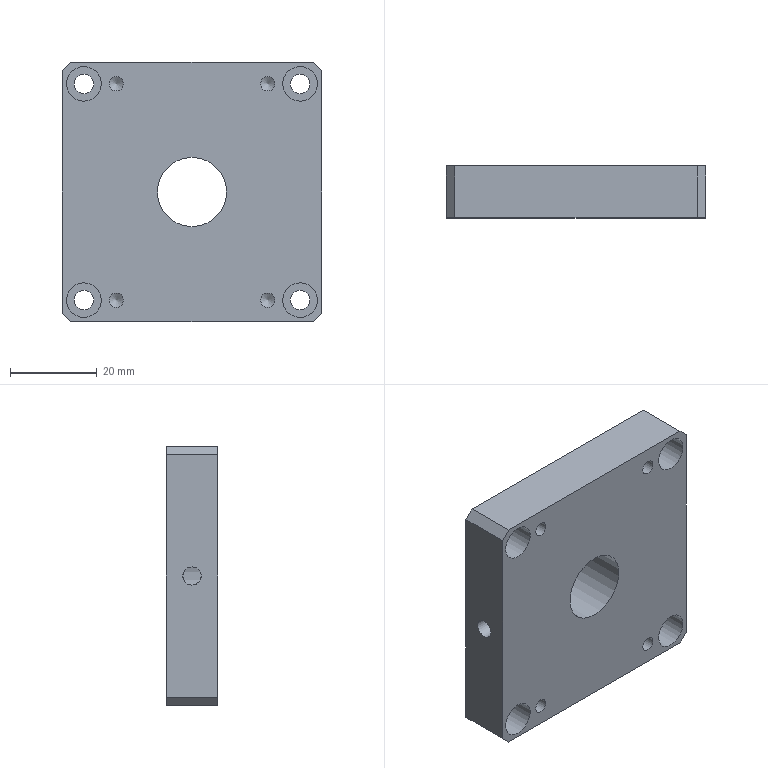Part | NX | 1 solid | 42 faces | box 60 x 12 x 60 mm | volume 38260 mm3 | plane 18 | cylinder 17 | cone 7 | commonest cylinder face diameters 3.3 x4 4.5 x4 8 x4 2 x3 4.2 x1 16 x1
STEP:
#1=CARTESIAN_POINT('',(-30.,6.,2.1));
#2=VERTEX_POINT('',#1);
#3=CARTESIAN_POINT('',(-30.,6.,0.));
#4=DIRECTION('',(-1.,0.,0.));
#5=DIRECTION('',(0.,0.,1.));
#6=AXIS2_PLACEMENT_3D('',#3,#4,#5);
#7=CIRCLE('',#6,2.1);
#8=EDGE_CURVE('',#2,#2,#7,.T.);
#9=ORIENTED_EDGE('',*,*,#8,.T.);
#10=EDGE_LOOP('',(#9));
#11=FACE_BOUND('',#10,.T.);
#12=CARTESIAN_POINT('',(-7.728,6.358,-2.069));
#13=VERTEX_POINT('',#12);
#14=CARTESIAN_POINT('',(-7.932,7.9,-1.344));
#15=CARTESIAN_POINT('',(-7.661,6.398,-2.294));
#16=CARTESIAN_POINT('',(-7.792,4.654,-1.898));
#17=CARTESIAN_POINT('',(-8.057,3.707,-0.4002));
#18=CARTESIAN_POINT('',(-7.932,4.101,1.346));
#19=CARTESIAN_POINT('',(-7.661,5.601,2.292));
#20=CARTESIAN_POINT('',(-7.791,7.344,1.9));
#21=CARTESIAN_POINT('',(-8.057,8.293,0.3983));
#22=CARTESIAN_POINT('',(-7.932,7.9,-1.344));
#23=CARTESIAN_POINT('',(-7.661,6.398,-2.294));
#24=CARTESIAN_POINT('',(-7.792,4.654,-1.898));
#25=B_SPLINE_CURVE_WITH_KNOTS('',3,(#14,#15,#16,#17,#18,#19,#20,#21,#22,#23,#24),.UNSPECIFIED.,.T.,.F.,(1,1,1,1,1,1,1,1,1,1,1,1,1,1,1),(-0.004946,-0.003297,-0.001649,0.,0.001649,0.003297,0.004946,0.006595,0.008243,0.009892,0.01154,0.01319,0.01484,0.01649,0.01814),.UNSPECIFIED.);
#26=EDGE_CURVE('',#13,#13,#25,.T.);
#27=ORIENTED_EDGE('',*,*,#26,.F.);
#28=EDGE_LOOP('',(#27));
#29=FACE_BOUND('',#28,.T.);
#30=CARTESIAN_POINT('',(-30.,6.,0.));
#31=DIRECTION('',(-1.,0.,0.));
#32=DIRECTION('',(0.,0.,1.));
#33=AXIS2_PLACEMENT_3D('',#30,#31,#32);
#34=CYLINDRICAL_SURFACE('',#33,2.1);
#35=ADVANCED_FACE('',(#11,#29),#34,.F.);
#36=CARTESIAN_POINT('',(0.,0.,-8.));
#37=VERTEX_POINT('',#36);
#38=CARTESIAN_POINT('',(0.,0.,0.));
#39=DIRECTION('',(0.,-1.,0.));
#40=DIRECTION('',(0.,0.,-1.));
#41=AXIS2_PLACEMENT_3D('',#38,#39,#40);
#42=CIRCLE('',#41,8.);
#43=EDGE_CURVE('',#37,#37,#42,.F.);
#44=ORIENTED_EDGE('',*,*,#43,.T.);
#45=EDGE_LOOP('',(#44));
#46=FACE_BOUND('',#45,.T.);
#47=CARTESIAN_POINT('',(-30.,0.,-28.));
#48=VERTEX_POINT('',#47);
#49=CARTESIAN_POINT('',(-30.,0.,28.));
#50=VERTEX_POINT('',#49);
#51=CARTESIAN_POINT('',(-30.,0.,30.));
#52=DIRECTION('',(0.,0.,1.));
#53=VECTOR('',#52,1000.);
#54=LINE('',#51,#53);
#55=EDGE_CURVE('',#48,#50,#54,.T.);
#56=ORIENTED_EDGE('',*,*,#55,.F.);
#57=CARTESIAN_POINT('',(-28.,0.,-30.));
#58=VERTEX_POINT('',#57);
#59=CARTESIAN_POINT('',(-29.,0.,-29.));
#60=DIRECTION('',(0.7071,0.,-0.7071));
#61=VECTOR('',#60,1000.);
#62=LINE('',#59,#61);
#63=EDGE_CURVE('',#48,#58,#62,.T.);
#64=ORIENTED_EDGE('',*,*,#63,.T.);
#65=CARTESIAN_POINT('',(28.,0.,-30.));
#66=VERTEX_POINT('',#65);
#67=CARTESIAN_POINT('',(-30.,0.,-30.));
#68=DIRECTION('',(-1.,0.,0.));
#69=VECTOR('',#68,1000.);
#70=LINE('',#67,#69);
#71=EDGE_CURVE('',#66,#58,#70,.T.);
#72=ORIENTED_EDGE('',*,*,#71,.F.);
#73=CARTESIAN_POINT('',(30.,0.,-28.));
#74=VERTEX_POINT('',#73);
#75=CARTESIAN_POINT('',(29.,0.,-29.));
#76=DIRECTION('',(0.7071,0.,0.7071));
#77=VECTOR('',#76,1000.);
#78=LINE('',#75,#77);
#79=EDGE_CURVE('',#66,#74,#78,.T.);
#80=ORIENTED_EDGE('',*,*,#79,.T.);
#81=CARTESIAN_POINT('',(30.,0.,28.));
#82=VERTEX_POINT('',#81);
#83=CARTESIAN_POINT('',(30.,0.,30.));
#84=DIRECTION('',(0.,0.,-1.));
#85=VECTOR('',#84,1000.);
#86=LINE('',#83,#85);
#87=EDGE_CURVE('',#82,#74,#86,.T.);
#88=ORIENTED_EDGE('',*,*,#87,.F.);
#89=CARTESIAN_POINT('',(28.,0.,30.));
#90=VERTEX_POINT('',#89);
#91=CARTESIAN_POINT('',(29.,0.,29.));
#92=DIRECTION('',(-0.7071,0.,0.7071));
#93=VECTOR('',#92,1000.);
#94=LINE('',#91,#93);
#95=EDGE_CURVE('',#82,#90,#94,.T.);
#96=ORIENTED_EDGE('',*,*,#95,.T.);
#97=CARTESIAN_POINT('',(-28.,0.,30.));
#98=VERTEX_POINT('',#97);
#99=CARTESIAN_POINT('',(-30.,0.,30.));
#100=DIRECTION('',(1.,0.,0.));
#101=VECTOR('',#100,1000.);
#102=LINE('',#99,#101);
#103=EDGE_CURVE('',#98,#90,#102,.T.);
#104=ORIENTED_EDGE('',*,*,#103,.F.);
#105=CARTESIAN_POINT('',(-29.,0.,29.));
#106=DIRECTION('',(-0.7071,0.,-0.7071));
#107=VECTOR('',#106,1000.);
#108=LINE('',#105,#107);
#109=EDGE_CURVE('',#98,#50,#108,.T.);
#110=ORIENTED_EDGE('',*,*,#109,.T.);
#111=EDGE_LOOP('',(#56,#64,#72,#80,#88,#96,#104,#110));
#112=FACE_BOUND('',#111,.T.);
#113=CARTESIAN_POINT('',(25.,0.,21.));
#114=VERTEX_POINT('',#113);
#115=CARTESIAN_POINT('',(25.,0.,25.));
#116=DIRECTION('',(0.,-1.,0.));
#117=DIRECTION('',(0.,0.,-1.));
#118=AXIS2_PLACEMENT_3D('',#115,#116,#117);
#119=CIRCLE('',#118,4.);
#120=EDGE_CURVE('',#114,#114,#119,.T.);
#121=ORIENTED_EDGE('',*,*,#120,.F.);
#122=EDGE_LOOP('',(#121));
#123=FACE_BOUND('',#122,.T.);
#124=CARTESIAN_POINT('',(25.,0.,-29.));
#125=VERTEX_POINT('',#124);
#126=CARTESIAN_POINT('',(25.,0.,-25.));
#127=DIRECTION('',(0.,-1.,0.));
#128=DIRECTION('',(0.,0.,-1.));
#129=AXIS2_PLACEMENT_3D('',#126,#127,#128);
#130=CIRCLE('',#129,4.);
#131=EDGE_CURVE('',#125,#125,#130,.T.);
#132=ORIENTED_EDGE('',*,*,#131,.F.);
#133=EDGE_LOOP('',(#132));
#134=FACE_BOUND('',#133,.T.);
#135=CARTESIAN_POINT('',(-25.,0.,-29.));
#136=VERTEX_POINT('',#135);
#137=CARTESIAN_POINT('',(-25.,0.,-25.));
#138=DIRECTION('',(0.,-1.,0.));
#139=DIRECTION('',(0.,0.,-1.));
#140=AXIS2_PLACEMENT_3D('',#137,#138,#139);
#141=CIRCLE('',#140,4.);
#142=EDGE_CURVE('',#136,#136,#141,.T.);
#143=ORIENTED_EDGE('',*,*,#142,.F.);
#144=EDGE_LOOP('',(#143));
#145=FACE_BOUND('',#144,.T.);
#146=CARTESIAN_POINT('',(-25.,0.,21.));
#147=VERTEX_POINT('',#146);
#148=CARTESIAN_POINT('',(-25.,0.,25.));
#149=DIRECTION('',(0.,-1.,0.));
#150=DIRECTION('',(0.,0.,-1.));
#151=AXIS2_PLACEMENT_3D('',#148,#149,#150);
#152=CIRCLE('',#151,4.);
#153=EDGE_CURVE('',#147,#147,#152,.T.);
#154=ORIENTED_EDGE('',*,*,#153,.F.);
#155=EDGE_LOOP('',(#154));
#156=FACE_BOUND('',#155,.T.);
#157=CARTESIAN_POINT('',(17.5,0.,23.35));
#158=VERTEX_POINT('',#157);
#159=CARTESIAN_POINT('',(17.5,0.,25.));
#160=DIRECTION('',(0.,-1.,0.));
#161=DIRECTION('',(0.,0.,-1.));
#162=AXIS2_PLACEMENT_3D('',#159,#160,#161);
#163=CIRCLE('',#162,1.65);
#164=EDGE_CURVE('',#158,#158,#163,.T.);
#165=ORIENTED_EDGE('',*,*,#164,.F.);
#166=EDGE_LOOP('',(#165));
#167=FACE_BOUND('',#166,.T.);
#168=CARTESIAN_POINT('',(17.5,0.,-26.65));
#169=VERTEX_POINT('',#168);
#170=CARTESIAN_POINT('',(17.5,0.,-25.));
#171=DIRECTION('',(0.,-1.,0.));
#172=DIRECTION('',(0.,0.,-1.));
#173=AXIS2_PLACEMENT_3D('',#170,#171,#172);
#174=CIRCLE('',#173,1.65);
#175=EDGE_CURVE('',#169,#169,#174,.T.);
#176=ORIENTED_EDGE('',*,*,#175,.F.);
#177=EDGE_LOOP('',(#176));
#178=FACE_BOUND('',#177,.T.);
#179=CARTESIAN_POINT('',(-17.5,0.,-26.65));
#180=VERTEX_POINT('',#179);
#181=CARTESIAN_POINT('',(-17.5,0.,-25.));
#182=DIRECTION('',(0.,-1.,0.));
#183=DIRECTION('',(0.,0.,-1.));
#184=AXIS2_PLACEMENT_3D('',#181,#182,#183);
#185=CIRCLE('',#184,1.65);
#186=EDGE_CURVE('',#180,#180,#185,.T.);
#187=ORIENTED_EDGE('',*,*,#186,.F.);
#188=EDGE_LOOP('',(#187));
#189=FACE_BOUND('',#188,.T.);
#190=CARTESIAN_POINT('',(-17.5,0.,23.35));
#191=VERTEX_POINT('',#190);
#192=CARTESIAN_POINT('',(-17.5,0.,25.));
#193=DIRECTION('',(0.,-1.,0.));
#194=DIRECTION('',(0.,0.,-1.));
#195=AXIS2_PLACEMENT_3D('',#192,#193,#194);
#196=CIRCLE('',#195,1.65);
#197=EDGE_CURVE('',#191,#191,#196,.T.);
#198=ORIENTED_EDGE('',*,*,#197,.F.);
#199=EDGE_LOOP('',(#198));
#200=FACE_BOUND('',#199,.T.);
#201=CARTESIAN_POINT('',(0.,0.,0.));
#202=DIRECTION('',(0.,-1.,0.));
#203=DIRECTION('',(0.,0.,-1.));
#204=AXIS2_PLACEMENT_3D('',#201,#202,#203);
#205=PLANE('',#204);
#206=ADVANCED_FACE('',(#46,#112,#123,#134,#145,#156,#167,#178,#189,#200),#205,.T.);
#207=CARTESIAN_POINT('',(0.,7.,-24.));
#208=VERTEX_POINT('',#207);
#209=CARTESIAN_POINT('',(0.,7.,-25.));
#210=DIRECTION('',(0.,1.,0.));
#211=DIRECTION('',(0.,0.,1.));
#212=AXIS2_PLACEMENT_3D('',#209,#210,#211);
#213=CIRCLE('',#212,1.);
#214=EDGE_CURVE('',#208,#208,#213,.T.);
#215=ORIENTED_EDGE('',*,*,#214,.T.);
#216=EDGE_LOOP('',(#215));
#217=FACE_BOUND('',#216,.T.);
#218=CARTESIAN_POINT('',(0.,6.399,-25.));
#219=VERTEX_POINT('',#218);
#220=VERTEX_LOOP('',#219);
#221=FACE_BOUND('',#220,.T.);
#222=CARTESIAN_POINT('',(0.,7.,-25.));
#223=DIRECTION('',(0.,1.,0.));
#224=DIRECTION('',(0.,0.,1.));
#225=AXIS2_PLACEMENT_3D('',#222,#223,#224);
#226=CONICAL_SURFACE('',#225,1.,1.03);
#227=ADVANCED_FACE('',(#217,#221),#226,.F.);
#228=CARTESIAN_POINT('',(1.,7.,24.5));
#229=VERTEX_POINT('',#228);
#230=CARTESIAN_POINT('',(0.,6.399,24.5));
#231=VERTEX_POINT('',#230);
#232=CARTESIAN_POINT('',(0.,6.399,24.5));
#233=DIRECTION('',(-0.8572,-0.515,0.));
#234=VECTOR('',#233,1000.);
#235=LINE('',#232,#234);
#236=EDGE_CURVE('',#229,#231,#235,.T.);
#237=ORIENTED_EDGE('',*,*,#236,.F.);
#238=CARTESIAN_POINT('',(-1.,7.,24.5));
#239=VERTEX_POINT('',#238);
#240=CARTESIAN_POINT('',(0.,7.,24.5));
#241=DIRECTION('',(0.,1.,0.));
#242=DIRECTION('',(0.,0.,1.));
#243=AXIS2_PLACEMENT_3D('',#240,#241,#242);
#244=CIRCLE('',#243,1.);
#245=EDGE_CURVE('',#229,#239,#244,.T.);
#246=ORIENTED_EDGE('',*,*,#245,.T.);
#247=CARTESIAN_POINT('',(0.,6.399,24.5));
#248=DIRECTION('',(-0.8572,0.515,0.));
#249=VECTOR('',#248,1000.);
#250=LINE('',#247,#249);
#251=EDGE_CURVE('',#231,#239,#250,.T.);
#252=ORIENTED_EDGE('',*,*,#251,.F.);
#253=EDGE_LOOP('',(#237,#246,#252));
#254=FACE_BOUND('',#253,.T.);
#255=CARTESIAN_POINT('',(0.,7.,24.5));
#256=DIRECTION('',(0.,1.,0.));
#257=DIRECTION('',(0.,0.,1.));
#258=AXIS2_PLACEMENT_3D('',#255,#256,#257);
#259=CONICAL_SURFACE('',#258,1.,1.03);
#260=ADVANCED_FACE('',(#254),#259,.F.);
#261=CARTESIAN_POINT('',(-1.,7.,25.5));
#262=VERTEX_POINT('',#261);
#263=CARTESIAN_POINT('',(-1.,7.,25.5));
#264=DIRECTION('',(0.,0.,-1.));
#265=VECTOR('',#264,1000.);
#266=LINE('',#263,#265);
#267=EDGE_CURVE('',#262,#239,#266,.T.);
#268=ORIENTED_EDGE('',*,*,#267,.F.);
#269=CARTESIAN_POINT('',(0.,6.399,25.5));
#270=VERTEX_POINT('',#269);
#271=CARTESIAN_POINT('',(0.,6.399,25.5));
#272=DIRECTION('',(0.8572,-0.515,0.));
#273=VECTOR('',#272,1000.);
#274=LINE('',#271,#273);
#275=EDGE_CURVE('',#262,#270,#274,.T.);
#276=ORIENTED_EDGE('',*,*,#275,.T.);
#277=CARTESIAN_POINT('',(0.,6.399,25.5));
#278=DIRECTION('',(0.,0.,-1.));
#279=VECTOR('',#278,1000.);
#280=LINE('',#277,#279);
#281=EDGE_CURVE('',#270,#231,#280,.T.);
#282=ORIENTED_EDGE('',*,*,#281,.T.);
#283=ORIENTED_EDGE('',*,*,#251,.T.);
#284=EDGE_LOOP('',(#268,#276,#282,#283));
#285=FACE_BOUND('',#284,.T.);
#286=CARTESIAN_POINT('',(0.,6.399,25.5));
#287=DIRECTION('',(-0.515,-0.8572,0.));
#288=DIRECTION('',(0.8572,-0.515,0.));
#289=AXIS2_PLACEMENT_3D('',#286,#287,#288);
#290=PLANE('',#289);
#291=ADVANCED_FACE('',(#285),#290,.F.);
#292=CARTESIAN_POINT('',(1.,7.,25.5));
#293=VERTEX_POINT('',#292);
#294=CARTESIAN_POINT('',(0.,6.399,25.5));
#295=DIRECTION('',(-0.8572,-0.515,0.));
#296=VECTOR('',#295,1000.);
#297=LINE('',#294,#296);
#298=EDGE_CURVE('',#293,#270,#297,.T.);
#299=ORIENTED_EDGE('',*,*,#298,.T.);
#300=ORIENTED_EDGE('',*,*,#275,.F.);
#301=CARTESIAN_POINT('',(0.,7.,25.5));
#302=DIRECTION('',(0.,1.,0.));
#303=DIRECTION('',(0.,0.,1.));
#304=AXIS2_PLACEMENT_3D('',#301,#302,#303);
#305=CIRCLE('',#304,1.);
#306=EDGE_CURVE('',#262,#293,#305,.T.);
#307=ORIENTED_EDGE('',*,*,#306,.T.);
#308=EDGE_LOOP('',(#299,#300,#307));
#309=FACE_BOUND('',#308,.T.);
#310=CARTESIAN_POINT('',(0.,7.,25.5));
#311=DIRECTION('',(0.,1.,0.));
#312=DIRECTION('',(0.,0.,1.));
#313=AXIS2_PLACEMENT_3D('',#310,#311,#312);
#314=CONICAL_SURFACE('',#313,1.,1.03);
#315=ADVANCED_FACE('',(#309),#314,.F.);
#316=CARTESIAN_POINT('',(1.,7.,25.5));
#317=DIRECTION('',(0.,0.,-1.));
#318=VECTOR('',#317,1000.);
#319=LINE('',#316,#318);
#320=EDGE_CURVE('',#293,#229,#319,.T.);
#321=ORIENTED_EDGE('',*,*,#320,.T.);
#322=ORIENTED_EDGE('',*,*,#236,.T.);
#323=ORIENTED_EDGE('',*,*,#281,.F.);
#324=ORIENTED_EDGE('',*,*,#298,.F.);
#325=EDGE_LOOP('',(#321,#322,#323,#324));
#326=FACE_BOUND('',#325,.T.);
#327=CARTESIAN_POINT('',(0.,6.399,25.5));
#328=DIRECTION('',(0.515,-0.8572,0.));
#329=DIRECTION('',(0.8572,0.515,0.));
#330=AXIS2_PLACEMENT_3D('',#327,#328,#329);
#331=PLANE('',#330);
#332=ADVANCED_FACE('',(#326),#331,.F.);
#333=ORIENTED_EDGE('',*,*,#214,.F.);
#334=EDGE_LOOP('',(#333));
#335=FACE_BOUND('',#334,.T.);
#336=CARTESIAN_POINT('',(0.,12.,-24.));
#337=VERTEX_POINT('',#336);
#338=CARTESIAN_POINT('',(0.,12.,-25.));
#339=DIRECTION('',(0.,1.,0.));
#340=DIRECTION('',(0.,0.,1.));
#341=AXIS2_PLACEMENT_3D('',#338,#339,#340);
#342=CIRCLE('',#341,1.);
#343=EDGE_CURVE('',#337,#337,#342,.T.);
#344=ORIENTED_EDGE('',*,*,#343,.T.);
#345=EDGE_LOOP('',(#344));
#346=FACE_BOUND('',#345,.T.);
#347=CARTESIAN_POINT('',(0.,12.,-25.));
#348=DIRECTION('',(0.,1.,0.));
#349=DIRECTION('',(0.,0.,1.));
#350=AXIS2_PLACEMENT_3D('',#347,#348,#349);
#351=CYLINDRICAL_SURFACE('',#350,1.);
#352=ADVANCED_FACE('',(#335,#346),#351,.F.);
#353=ORIENTED_EDGE('',*,*,#245,.F.);
#354=CARTESIAN_POINT('',(1.,12.,24.5));
#355=VERTEX_POINT('',#354);
#356=CARTESIAN_POINT('',(1.,7.,24.5));
#357=DIRECTION('',(0.,-1.,0.));
#358=VECTOR('',#357,1000.);
#359=LINE('',#356,#358);
#360=EDGE_CURVE('',#355,#229,#359,.T.);
#361=ORIENTED_EDGE('',*,*,#360,.F.);
#362=CARTESIAN_POINT('',(-1.,12.,24.5));
#363=VERTEX_POINT('',#362);
#364=CARTESIAN_POINT('',(0.,12.,24.5));
#365=DIRECTION('',(0.,1.,0.));
#366=DIRECTION('',(0.,0.,1.));
#367=AXIS2_PLACEMENT_3D('',#364,#365,#366);
#368=CIRCLE('',#367,1.);
#369=EDGE_CURVE('',#355,#363,#368,.T.);
#370=ORIENTED_EDGE('',*,*,#369,.T.);
#371=CARTESIAN_POINT('',(-1.,12.,24.5));
#372=DIRECTION('',(0.,1.,0.));
#373=VECTOR('',#372,1000.);
#374=LINE('',#371,#373);
#375=EDGE_CURVE('',#239,#363,#374,.T.);
#376=ORIENTED_EDGE('',*,*,#375,.F.);
#377=EDGE_LOOP('',(#353,#361,#370,#376));
#378=FACE_BOUND('',#377,.T.);
#379=CARTESIAN_POINT('',(0.,12.,24.5));
#380=DIRECTION('',(0.,1.,0.));
#381=DIRECTION('',(0.,0.,1.));
#382=AXIS2_PLACEMENT_3D('',#379,#380,#381);
#383=CYLINDRICAL_SURFACE('',#382,1.);
#384=ADVANCED_FACE('',(#378),#383,.F.);
#385=CARTESIAN_POINT('',(-1.,12.,25.5));
#386=VERTEX_POINT('',#385);
#387=CARTESIAN_POINT('',(-1.,12.,25.5));
#388=DIRECTION('',(0.,0.,-1.));
#389=VECTOR('',#388,1000.);
#390=LINE('',#387,#389);
#391=EDGE_CURVE('',#386,#363,#390,.T.);
#392=ORIENTED_EDGE('',*,*,#391,.F.);
#393=CARTESIAN_POINT('',(-1.,12.,25.5));
#394=DIRECTION('',(0.,-1.,0.));
#395=VECTOR('',#394,1000.);
#396=LINE('',#393,#395);
#397=EDGE_CURVE('',#386,#262,#396,.T.);
#398=ORIENTED_EDGE('',*,*,#397,.T.);
#399=ORIENTED_EDGE('',*,*,#267,.T.);
#400=ORIENTED_EDGE('',*,*,#375,.T.);
#401=EDGE_LOOP('',(#392,#398,#399,#400));
#402=FACE_BOUND('',#401,.T.);
#403=CARTESIAN_POINT('',(-1.,12.,25.5));
#404=DIRECTION('',(-1.,0.,0.));
#405=DIRECTION('',(0.,0.,1.));
#406=AXIS2_PLACEMENT_3D('',#403,#404,#405);
#407=PLANE('',#406);
#408=ADVANCED_FACE('',(#402),#407,.F.);
#409=ORIENTED_EDGE('',*,*,#306,.F.);
#410=ORIENTED_EDGE('',*,*,#397,.F.);
#411=CARTESIAN_POINT('',(1.,12.,25.5));
#412=VERTEX_POINT('',#411);
#413=CARTESIAN_POINT('',(0.,12.,25.5));
#414=DIRECTION('',(0.,1.,0.));
#415=DIRECTION('',(0.,0.,1.));
#416=AXIS2_PLACEMENT_3D('',#413,#414,#415);
#417=CIRCLE('',#416,1.);
#418=EDGE_CURVE('',#386,#412,#417,.T.);
#419=ORIENTED_EDGE('',*,*,#418,.T.);
#420=CARTESIAN_POINT('',(1.,7.,25.5));
#421=DIRECTION('',(0.,-1.,0.));
#422=VECTOR('',#421,1000.);
#423=LINE('',#420,#422);
#424=EDGE_CURVE('',#412,#293,#423,.T.);
#425=ORIENTED_EDGE('',*,*,#424,.T.);
#426=EDGE_LOOP('',(#409,#410,#419,#425));
#427=FACE_BOUND('',#426,.T.);
#428=CARTESIAN_POINT('',(0.,12.,25.5));
#429=DIRECTION('',(0.,1.,0.));
#430=DIRECTION('',(0.,0.,1.));
#431=AXIS2_PLACEMENT_3D('',#428,#429,#430);
#432=CYLINDRICAL_SURFACE('',#431,1.);
#433=ADVANCED_FACE('',(#427),#432,.F.);
#434=CARTESIAN_POINT('',(1.,12.,25.5));
#435=DIRECTION('',(0.,0.,-1.));
#436=VECTOR('',#435,1000.);
#437=LINE('',#434,#436);
#438=EDGE_CURVE('',#412,#355,#437,.T.);
#439=ORIENTED_EDGE('',*,*,#438,.T.);
#440=ORIENTED_EDGE('',*,*,#360,.T.);
#441=ORIENTED_EDGE('',*,*,#320,.F.);
#442=ORIENTED_EDGE('',*,*,#424,.F.);
#443=EDGE_LOOP('',(#439,#440,#441,#442));
#444=FACE_BOUND('',#443,.T.);
#445=CARTESIAN_POINT('',(1.,7.,25.5));
#446=DIRECTION('',(1.,0.,0.));
#447=DIRECTION('',(0.,1.,0.));
#448=AXIS2_PLACEMENT_3D('',#445,#446,#447);
#449=PLANE('',#448);
#450=ADVANCED_FACE('',(#444),#449,.F.);
#451=CARTESIAN_POINT('',(-25.,7.,22.75));
#452=VERTEX_POINT('',#451);
#453=CARTESIAN_POINT('',(-25.,7.,25.));
#454=DIRECTION('',(0.,-1.,0.));
#455=DIRECTION('',(0.,0.,-1.));
#456=AXIS2_PLACEMENT_3D('',#453,#454,#455);
#457=CIRCLE('',#456,2.25);
#458=EDGE_CURVE('',#452,#452,#457,.T.);
#459=ORIENTED_EDGE('',*,*,#458,.T.);
#460=EDGE_LOOP('',(#459));
#461=FACE_BOUND('',#460,.T.);
#462=CARTESIAN_POINT('',(-25.,12.,22.75));
#463=VERTEX_POINT('',#462);
#464=CARTESIAN_POINT('',(-25.,12.,25.));
#465=DIRECTION('',(0.,-1.,0.));
#466=DIRECTION('',(0.,0.,-1.));
#467=AXIS2_PLACEMENT_3D('',#464,#465,#466);
#468=CIRCLE('',#467,2.25);
#469=EDGE_CURVE('',#463,#463,#468,.T.);
#470=ORIENTED_EDGE('',*,*,#469,.F.);
#471=EDGE_LOOP('',(#470));
#472=FACE_BOUND('',#471,.T.);
#473=CARTESIAN_POINT('',(-25.,0.,25.));
#474=DIRECTION('',(0.,-1.,0.));
#475=DIRECTION('',(0.,0.,-1.));
#476=AXIS2_PLACEMENT_3D('',#473,#474,#475);
#477=CYLINDRICAL_SURFACE('',#476,2.25);
#478=ADVANCED_FACE('',(#461,#472),#477,.F.);
#479=CARTESIAN_POINT('',(-25.,7.,-22.75));
#480=VERTEX_POINT('',#479);
#481=CARTESIAN_POINT('',(-25.,7.,-25.));
#482=DIRECTION('',(0.,-1.,0.));
#483=DIRECTION('',(0.,0.,1.));
#484=AXIS2_PLACEMENT_3D('',#481,#482,#483);
#485=CIRCLE('',#484,2.25);
#486=EDGE_CURVE('',#480,#480,#485,.T.);
#487=ORIENTED_EDGE('',*,*,#486,.T.);
#488=EDGE_LOOP('',(#487));
#489=FACE_BOUND('',#488,.T.);
#490=CARTESIAN_POINT('',(-25.,12.,-27.25));
#491=VERTEX_POINT('',#490);
#492=CARTESIAN_POINT('',(-25.,12.,-25.));
#493=DIRECTION('',(0.,-1.,0.));
#494=DIRECTION('',(0.,0.,-1.));
#495=AXIS2_PLACEMENT_3D('',#492,#493,#494);
#496=CIRCLE('',#495,2.25);
#497=EDGE_CURVE('',#491,#491,#496,.T.);
#498=ORIENTED_EDGE('',*,*,#497,.F.);
#499=EDGE_LOOP('',(#498));
#500=FACE_BOUND('',#499,.T.);
#501=CARTESIAN_POINT('',(-25.,0.,-25.));
#502=DIRECTION('',(0.,-1.,0.));
#503=DIRECTION('',(0.,0.,-1.));
#504=AXIS2_PLACEMENT_3D('',#501,#502,#503);
#505=CYLINDRICAL_SURFACE('',#504,2.25);
#506=ADVANCED_FACE('',(#489,#500),#505,.F.);
#507=CARTESIAN_POINT('',(25.,7.,-22.75));
#508=VERTEX_POINT('',#507);
#509=CARTESIAN_POINT('',(25.,7.,-25.));
#510=DIRECTION('',(0.,-1.,0.));
#511=DIRECTION('',(0.,0.,1.));
#512=AXIS2_PLACEMENT_3D('',#509,#510,#511);
#513=CIRCLE('',#512,2.25);
#514=EDGE_CURVE('',#508,#508,#513,.T.);
#515=ORIENTED_EDGE('',*,*,#514,.T.);
#516=EDGE_LOOP('',(#515));
#517=FACE_BOUND('',#516,.T.);
#518=CARTESIAN_POINT('',(25.,12.,-27.25));
#519=VERTEX_POINT('',#518);
#520=CARTESIAN_POINT('',(25.,12.,-25.));
#521=DIRECTION('',(0.,-1.,0.));
#522=DIRECTION('',(0.,0.,-1.));
#523=AXIS2_PLACEMENT_3D('',#520,#521,#522);
#524=CIRCLE('',#523,2.25);
#525=EDGE_CURVE('',#519,#519,#524,.T.);
#526=ORIENTED_EDGE('',*,*,#525,.F.);
#527=EDGE_LOOP('',(#526));
#528=FACE_BOUND('',#527,.T.);
#529=CARTESIAN_POINT('',(25.,0.,-25.));
#530=DIRECTION('',(0.,-1.,0.));
#531=DIRECTION('',(0.,0.,-1.));
#532=AXIS2_PLACEMENT_3D('',#529,#530,#531);
#533=CYLINDRICAL_SURFACE('',#532,2.25);
#534=ADVANCED_FACE('',(#517,#528),#533,.F.);
#535=CARTESIAN_POINT('',(25.,7.,27.25));
#536=VERTEX_POINT('',#535);
#537=CARTESIAN_POINT('',(25.,7.,25.));
#538=DIRECTION('',(0.,-1.,0.));
#539=DIRECTION('',(0.,0.,1.));
#540=AXIS2_PLACEMENT_3D('',#537,#538,#539);
#541=CIRCLE('',#540,2.25);
#542=EDGE_CURVE('',#536,#536,#541,.T.);
#543=ORIENTED_EDGE('',*,*,#542,.T.);
#544=EDGE_LOOP('',(#543));
#545=FACE_BOUND('',#544,.T.);
#546=CARTESIAN_POINT('',(25.,12.,22.75));
#547=VERTEX_POINT('',#546);
#548=CARTESIAN_POINT('',(25.,12.,25.));
#549=DIRECTION('',(0.,-1.,0.));
#550=DIRECTION('',(0.,0.,-1.));
#551=AXIS2_PLACEMENT_3D('',#548,#549,#550);
#552=CIRCLE('',#551,2.25);
#553=EDGE_CURVE('',#547,#547,#552,.T.);
#554=ORIENTED_EDGE('',*,*,#553,.F.);
#555=EDGE_LOOP('',(#554));
#556=FACE_BOUND('',#555,.T.);
#557=CARTESIAN_POINT('',(25.,0.,25.));
#558=DIRECTION('',(0.,-1.,0.));
#559=DIRECTION('',(0.,0.,-1.));
#560=AXIS2_PLACEMENT_3D('',#557,#558,#559);
#561=CYLINDRICAL_SURFACE('',#560,2.25);
#562=ADVANCED_FACE('',(#545,#556),#561,.F.);
#563=CARTESIAN_POINT('',(-17.5,11.091,25.));
#564=VERTEX_POINT('',#563);
#565=VERTEX_LOOP('',#564);
#566=FACE_BOUND('',#565,.T.);
#567=CARTESIAN_POINT('',(-17.5,10.1,23.35));
#568=VERTEX_POINT('',#567);
#569=CARTESIAN_POINT('',(-17.5,10.1,25.));
#570=DIRECTION('',(0.,-1.,0.));
#571=DIRECTION('',(0.,0.,-1.));
#572=AXIS2_PLACEMENT_3D('',#569,#570,#571);
#573=CIRCLE('',#572,1.65);
#574=EDGE_CURVE('',#568,#568,#573,.T.);
#575=ORIENTED_EDGE('',*,*,#574,.T.);
#576=EDGE_LOOP('',(#575));
#577=FACE_BOUND('',#576,.T.);
#578=CARTESIAN_POINT('',(-17.5,10.1,25.));
#579=DIRECTION('',(0.,-1.,0.));
#580=DIRECTION('',(0.,0.,-1.));
#581=AXIS2_PLACEMENT_3D('',#578,#579,#580);
#582=CONICAL_SURFACE('',#581,1.65,1.03);
#583=ADVANCED_FACE('',(#566,#577),#582,.F.);
#584=CARTESIAN_POINT('',(-17.5,11.091,-25.));
#585=VERTEX_POINT('',#584);
#586=VERTEX_LOOP('',#585);
#587=FACE_BOUND('',#586,.T.);
#588=CARTESIAN_POINT('',(-17.5,10.1,-26.65));
#589=VERTEX_POINT('',#588);
#590=CARTESIAN_POINT('',(-17.5,10.1,-25.));
#591=DIRECTION('',(0.,-1.,0.));
#592=DIRECTION('',(0.,0.,-1.));
#593=AXIS2_PLACEMENT_3D('',#590,#591,#592);
#594=CIRCLE('',#593,1.65);
#595=EDGE_CURVE('',#589,#589,#594,.T.);
#596=ORIENTED_EDGE('',*,*,#595,.T.);
#597=EDGE_LOOP('',(#596));
#598=FACE_BOUND('',#597,.T.);
#599=CARTESIAN_POINT('',(-17.5,10.1,-25.));
#600=DIRECTION('',(0.,-1.,0.));
#601=DIRECTION('',(0.,0.,-1.));
#602=AXIS2_PLACEMENT_3D('',#599,#600,#601);
#603=CONICAL_SURFACE('',#602,1.65,1.03);
#604=ADVANCED_FACE('',(#587,#598),#603,.F.);
#605=CARTESIAN_POINT('',(17.5,11.091,-25.));
#606=VERTEX_POINT('',#605);
#607=VERTEX_LOOP('',#606);
#608=FACE_BOUND('',#607,.T.);
#609=CARTESIAN_POINT('',(17.5,10.1,-26.65));
#610=VERTEX_POINT('',#609);
#611=CARTESIAN_POINT('',(17.5,10.1,-25.));
#612=DIRECTION('',(0.,-1.,0.));
#613=DIRECTION('',(0.,0.,-1.));
#614=AXIS2_PLACEMENT_3D('',#611,#612,#613);
#615=CIRCLE('',#614,1.65);
#616=EDGE_CURVE('',#610,#610,#615,.T.);
#617=ORIENTED_EDGE('',*,*,#616,.T.);
#618=EDGE_LOOP('',(#617));
#619=FACE_BOUND('',#618,.T.);
#620=CARTESIAN_POINT('',(17.5,10.1,-25.));
#621=DIRECTION('',(0.,-1.,0.));
#622=DIRECTION('',(0.,0.,-1.));
#623=AXIS2_PLACEMENT_3D('',#620,#621,#622);
#624=CONICAL_SURFACE('',#623,1.65,1.03);
#625=ADVANCED_FACE('',(#608,#619),#624,.F.);
#626=CARTESIAN_POINT('',(17.5,11.091,25.));
#627=VERTEX_POINT('',#626);
#628=VERTEX_LOOP('',#627);
#629=FACE_BOUND('',#628,.T.);
#630=CARTESIAN_POINT('',(17.5,10.1,23.35));
#631=VERTEX_POINT('',#630);
#632=CARTESIAN_POINT('',(17.5,10.1,25.));
#633=DIRECTION('',(0.,-1.,0.));
#634=DIRECTION('',(0.,0.,-1.));
#635=AXIS2_PLACEMENT_3D('',#632,#633,#634);
#636=CIRCLE('',#635,1.65);
#637=EDGE_CURVE('',#631,#631,#636,.T.);
#638=ORIENTED_EDGE('',*,*,#637,.T.);
#639=EDGE_LOOP('',(#638));
#640=FACE_BOUND('',#639,.T.);
#641=CARTESIAN_POINT('',(17.5,10.1,25.));
#642=DIRECTION('',(0.,-1.,0.));
#643=DIRECTION('',(0.,0.,-1.));
#644=AXIS2_PLACEMENT_3D('',#641,#642,#643);
#645=CONICAL_SURFACE('',#644,1.65,1.03);
#646=ADVANCED_FACE('',(#629,#640),#645,.F.);
#647=CARTESIAN_POINT('',(-25.,7.,21.));
#648=VERTEX_POINT('',#647);
#649=CARTESIAN_POINT('',(-25.,7.,25.));
#650=DIRECTION('',(0.,-1.,0.));
#651=DIRECTION('',(0.,0.,-1.));
#652=AXIS2_PLACEMENT_3D('',#649,#650,#651);
#653=CIRCLE('',#652,4.);
#654=EDGE_CURVE('',#648,#648,#653,.T.);
#655=ORIENTED_EDGE('',*,*,#654,.T.);
#656=EDGE_LOOP('',(#655));
#657=FACE_BOUND('',#656,.T.);
#658=ORIENTED_EDGE('',*,*,#458,.F.);
#659=EDGE_LOOP('',(#658));
#660=FACE_BOUND('',#659,.T.);
#661=CARTESIAN_POINT('',(-22.75,7.,25.));
#662=DIRECTION('',(0.,1.,0.));
#663=DIRECTION('',(0.,0.,1.));
#664=AXIS2_PLACEMENT_3D('',#661,#662,#663);
#665=PLANE('',#664);
#666=ADVANCED_FACE('',(#657,#660),#665,.F.);
#667=CARTESIAN_POINT('',(-25.,7.,-21.));
#668=VERTEX_POINT('',#667);
#669=CARTESIAN_POINT('',(-25.,7.,-25.));
#670=DIRECTION('',(0.,-1.,0.));
#671=DIRECTION('',(0.,0.,1.));
#672=AXIS2_PLACEMENT_3D('',#669,#670,#671);
#673=CIRCLE('',#672,4.);
#674=EDGE_CURVE('',#668,#668,#673,.T.);
#675=ORIENTED_EDGE('',*,*,#674,.T.);
#676=EDGE_LOOP('',(#675));
#677=FACE_BOUND('',#676,.T.);
#678=ORIENTED_EDGE('',*,*,#486,.F.);
#679=EDGE_LOOP('',(#678));
#680=FACE_BOUND('',#679,.T.);
#681=CARTESIAN_POINT('',(-22.75,7.,25.));
#682=DIRECTION('',(0.,1.,0.));
#683=DIRECTION('',(0.,0.,1.));
#684=AXIS2_PLACEMENT_3D('',#681,#682,#683);
#685=PLANE('',#684);
#686=ADVANCED_FACE('',(#677,#680),#685,.F.);
#687=CARTESIAN_POINT('',(25.,7.,-21.));
#688=VERTEX_POINT('',#687);
#689=CARTESIAN_POINT('',(25.,7.,-25.));
#690=DIRECTION('',(0.,-1.,0.));
#691=DIRECTION('',(0.,0.,1.));
#692=AXIS2_PLACEMENT_3D('',#689,#690,#691);
#693=CIRCLE('',#692,4.);
#694=EDGE_CURVE('',#688,#688,#693,.T.);
#695=ORIENTED_EDGE('',*,*,#694,.T.);
#696=EDGE_LOOP('',(#695));
#697=FACE_BOUND('',#696,.T.);
#698=ORIENTED_EDGE('',*,*,#514,.F.);
#699=EDGE_LOOP('',(#698));
#700=FACE_BOUND('',#699,.T.);
#701=CARTESIAN_POINT('',(-22.75,7.,25.));
#702=DIRECTION('',(0.,1.,0.));
#703=DIRECTION('',(0.,0.,1.));
#704=AXIS2_PLACEMENT_3D('',#701,#702,#703);
#705=PLANE('',#704);
#706=ADVANCED_FACE('',(#697,#700),#705,.F.);
#707=CARTESIAN_POINT('',(25.,7.,29.));
#708=VERTEX_POINT('',#707);
#709=CARTESIAN_POINT('',(25.,7.,25.));
#710=DIRECTION('',(0.,-1.,0.));
#711=DIRECTION('',(0.,0.,1.));
#712=AXIS2_PLACEMENT_3D('',#709,#710,#711);
#713=CIRCLE('',#712,4.);
#714=EDGE_CURVE('',#708,#708,#713,.T.);
#715=ORIENTED_EDGE('',*,*,#714,.T.);
#716=EDGE_LOOP('',(#715));
#717=FACE_BOUND('',#716,.T.);
#718=ORIENTED_EDGE('',*,*,#542,.F.);
#719=EDGE_LOOP('',(#718));
#720=FACE_BOUND('',#719,.T.);
#721=CARTESIAN_POINT('',(-22.75,7.,25.));
#722=DIRECTION('',(0.,1.,0.));
#723=DIRECTION('',(0.,0.,1.));
#724=AXIS2_PLACEMENT_3D('',#721,#722,#723);
#725=PLANE('',#724);
#726=ADVANCED_FACE('',(#717,#720),#725,.F.);
#727=CARTESIAN_POINT('',(0.,12.,-8.));
#728=VERTEX_POINT('',#727);
#729=CARTESIAN_POINT('',(0.,12.,0.));
#730=DIRECTION('',(0.,-1.,0.));
#731=DIRECTION('',(0.,0.,-1.));
#732=AXIS2_PLACEMENT_3D('',#729,#730,#731);
#733=CIRCLE('',#732,8.);
#734=EDGE_CURVE('',#728,#728,#733,.F.);
#735=ORIENTED_EDGE('',*,*,#734,.F.);
#736=EDGE_LOOP('',(#735));
#737=FACE_BOUND('',#736,.T.);
#738=CARTESIAN_POINT('',(28.,12.,-30.));
#739=VERTEX_POINT('',#738);
#740=CARTESIAN_POINT('',(-28.,12.,-30.));
#741=VERTEX_POINT('',#740);
#742=CARTESIAN_POINT('',(-30.,12.,-30.));
#743=DIRECTION('',(-1.,0.,0.));
#744=VECTOR('',#743,1000.);
#745=LINE('',#742,#744);
#746=EDGE_CURVE('',#739,#741,#745,.T.);
#747=ORIENTED_EDGE('',*,*,#746,.T.);
#748=CARTESIAN_POINT('',(-30.,12.,-28.));
#749=VERTEX_POINT('',#748);
#750=CARTESIAN_POINT('',(-30.,12.,-28.));
#751=DIRECTION('',(-0.7071,0.,0.7071));
#752=VECTOR('',#751,1000.);
#753=LINE('',#750,#752);
#754=EDGE_CURVE('',#741,#749,#753,.T.);
#755=ORIENTED_EDGE('',*,*,#754,.T.);
#756=CARTESIAN_POINT('',(-30.,12.,28.));
#757=VERTEX_POINT('',#756);
#758=CARTESIAN_POINT('',(-30.,12.,30.));
#759=DIRECTION('',(0.,0.,1.));
#760=VECTOR('',#759,1000.);
#761=LINE('',#758,#760);
#762=EDGE_CURVE('',#749,#757,#761,.T.);
#763=ORIENTED_EDGE('',*,*,#762,.T.);
#764=CARTESIAN_POINT('',(-28.,12.,30.));
#765=VERTEX_POINT('',#764);
#766=CARTESIAN_POINT('',(-28.,12.,30.));
#767=DIRECTION('',(0.7071,0.,0.7071));
#768=VECTOR('',#767,1000.);
#769=LINE('',#766,#768);
#770=EDGE_CURVE('',#757,#765,#769,.T.);
#771=ORIENTED_EDGE('',*,*,#770,.T.);
#772=CARTESIAN_POINT('',(28.,12.,30.));
#773=VERTEX_POINT('',#772);
#774=CARTESIAN_POINT('',(-30.,12.,30.));
#775=DIRECTION('',(1.,0.,0.));
#776=VECTOR('',#775,1000.);
#777=LINE('',#774,#776);
#778=EDGE_CURVE('',#765,#773,#777,.T.);
#779=ORIENTED_EDGE('',*,*,#778,.T.);
#780=CARTESIAN_POINT('',(30.,12.,28.));
#781=VERTEX_POINT('',#780);
#782=CARTESIAN_POINT('',(30.,12.,28.));
#783=DIRECTION('',(0.7071,0.,-0.7071));
#784=VECTOR('',#783,1000.);
#785=LINE('',#782,#784);
#786=EDGE_CURVE('',#773,#781,#785,.T.);
#787=ORIENTED_EDGE('',*,*,#786,.T.);
#788=CARTESIAN_POINT('',(30.,12.,-28.));
#789=VERTEX_POINT('',#788);
#790=CARTESIAN_POINT('',(30.,12.,30.));
#791=DIRECTION('',(0.,0.,-1.));
#792=VECTOR('',#791,1000.);
#793=LINE('',#790,#792);
#794=EDGE_CURVE('',#781,#789,#793,.T.);
#795=ORIENTED_EDGE('',*,*,#794,.T.);
#796=CARTESIAN_POINT('',(28.,12.,-30.));
#797=DIRECTION('',(-0.7071,0.,-0.7071));
#798=VECTOR('',#797,1000.);
#799=LINE('',#796,#798);
#800=EDGE_CURVE('',#789,#739,#799,.T.);
#801=ORIENTED_EDGE('',*,*,#800,.T.);
#802=EDGE_LOOP('',(#747,#755,#763,#771,#779,#787,#795,#801));
#803=FACE_BOUND('',#802,.T.);
#804=ORIENTED_EDGE('',*,*,#553,.T.);
#805=EDGE_LOOP('',(#804));
#806=FACE_BOUND('',#805,.T.);
#807=ORIENTED_EDGE('',*,*,#525,.T.);
#808=EDGE_LOOP('',(#807));
#809=FACE_BOUND('',#808,.T.);
#810=ORIENTED_EDGE('',*,*,#497,.T.);
#811=EDGE_LOOP('',(#810));
#812=FACE_BOUND('',#811,.T.);
#813=ORIENTED_EDGE('',*,*,#469,.T.);
#814=EDGE_LOOP('',(#813));
#815=FACE_BOUND('',#814,.T.);
#816=ORIENTED_EDGE('',*,*,#438,.F.);
#817=ORIENTED_EDGE('',*,*,#418,.F.);
#818=ORIENTED_EDGE('',*,*,#391,.T.);
#819=ORIENTED_EDGE('',*,*,#369,.F.);
#820=EDGE_LOOP('',(#816,#817,#818,#819));
#821=FACE_BOUND('',#820,.T.);
#822=ORIENTED_EDGE('',*,*,#343,.F.);
#823=EDGE_LOOP('',(#822));
#824=FACE_BOUND('',#823,.T.);
#825=CARTESIAN_POINT('',(0.,12.,0.));
#826=DIRECTION('',(0.,-1.,0.));
#827=DIRECTION('',(0.,0.,-1.));
#828=AXIS2_PLACEMENT_3D('',#825,#826,#827);
#829=PLANE('',#828);
#830=ADVANCED_FACE('',(#737,#803,#806,#809,#812,#815,#821,#824),#829,.F.);
#831=ORIENTED_EDGE('',*,*,#197,.T.);
#832=EDGE_LOOP('',(#831));
#833=FACE_BOUND('',#832,.T.);
#834=ORIENTED_EDGE('',*,*,#574,.F.);
#835=EDGE_LOOP('',(#834));
#836=FACE_BOUND('',#835,.T.);
#837=CARTESIAN_POINT('',(-17.5,0.,25.));
#838=DIRECTION('',(0.,-1.,0.));
#839=DIRECTION('',(0.,0.,-1.));
#840=AXIS2_PLACEMENT_3D('',#837,#838,#839);
#841=CYLINDRICAL_SURFACE('',#840,1.65);
#842=ADVANCED_FACE('',(#833,#836),#841,.F.);
#843=ORIENTED_EDGE('',*,*,#186,.T.);
#844=EDGE_LOOP('',(#843));
#845=FACE_BOUND('',#844,.T.);
#846=ORIENTED_EDGE('',*,*,#595,.F.);
#847=EDGE_LOOP('',(#846));
#848=FACE_BOUND('',#847,.T.);
#849=CARTESIAN_POINT('',(-17.5,0.,-25.));
#850=DIRECTION('',(0.,-1.,0.));
#851=DIRECTION('',(0.,0.,-1.));
#852=AXIS2_PLACEMENT_3D('',#849,#850,#851);
#853=CYLINDRICAL_SURFACE('',#852,1.65);
#854=ADVANCED_FACE('',(#845,#848),#853,.F.);
#855=ORIENTED_EDGE('',*,*,#175,.T.);
#856=EDGE_LOOP('',(#855));
#857=FACE_BOUND('',#856,.T.);
#858=ORIENTED_EDGE('',*,*,#616,.F.);
#859=EDGE_LOOP('',(#858));
#860=FACE_BOUND('',#859,.T.);
#861=CARTESIAN_POINT('',(17.5,0.,-25.));
#862=DIRECTION('',(0.,-1.,0.));
#863=DIRECTION('',(0.,0.,-1.));
#864=AXIS2_PLACEMENT_3D('',#861,#862,#863);
#865=CYLINDRICAL_SURFACE('',#864,1.65);
#866=ADVANCED_FACE('',(#857,#860),#865,.F.);
#867=ORIENTED_EDGE('',*,*,#164,.T.);
#868=EDGE_LOOP('',(#867));
#869=FACE_BOUND('',#868,.T.);
#870=ORIENTED_EDGE('',*,*,#637,.F.);
#871=EDGE_LOOP('',(#870));
#872=FACE_BOUND('',#871,.T.);
#873=CARTESIAN_POINT('',(17.5,0.,25.));
#874=DIRECTION('',(0.,-1.,0.));
#875=DIRECTION('',(0.,0.,-1.));
#876=AXIS2_PLACEMENT_3D('',#873,#874,#875);
#877=CYLINDRICAL_SURFACE('',#876,1.65);
#878=ADVANCED_FACE('',(#869,#872),#877,.F.);
#879=ORIENTED_EDGE('',*,*,#153,.T.);
#880=EDGE_LOOP('',(#879));
#881=FACE_BOUND('',#880,.T.);
#882=ORIENTED_EDGE('',*,*,#654,.F.);
#883=EDGE_LOOP('',(#882));
#884=FACE_BOUND('',#883,.T.);
#885=CARTESIAN_POINT('',(-25.,0.,25.));
#886=DIRECTION('',(0.,-1.,0.));
#887=DIRECTION('',(0.,0.,-1.));
#888=AXIS2_PLACEMENT_3D('',#885,#886,#887);
#889=CYLINDRICAL_SURFACE('',#888,4.);
#890=ADVANCED_FACE('',(#881,#884),#889,.F.);
#891=ORIENTED_EDGE('',*,*,#142,.T.);
#892=EDGE_LOOP('',(#891));
#893=FACE_BOUND('',#892,.T.);
#894=ORIENTED_EDGE('',*,*,#674,.F.);
#895=EDGE_LOOP('',(#894));
#896=FACE_BOUND('',#895,.T.);
#897=CARTESIAN_POINT('',(-25.,0.,-25.));
#898=DIRECTION('',(0.,-1.,0.));
#899=DIRECTION('',(0.,0.,-1.));
#900=AXIS2_PLACEMENT_3D('',#897,#898,#899);
#901=CYLINDRICAL_SURFACE('',#900,4.);
#902=ADVANCED_FACE('',(#893,#896),#901,.F.);
#903=ORIENTED_EDGE('',*,*,#131,.T.);
#904=EDGE_LOOP('',(#903));
#905=FACE_BOUND('',#904,.T.);
#906=ORIENTED_EDGE('',*,*,#694,.F.);
#907=EDGE_LOOP('',(#906));
#908=FACE_BOUND('',#907,.T.);
#909=CARTESIAN_POINT('',(25.,0.,-25.));
#910=DIRECTION('',(0.,-1.,0.));
#911=DIRECTION('',(0.,0.,-1.));
#912=AXIS2_PLACEMENT_3D('',#909,#910,#911);
#913=CYLINDRICAL_SURFACE('',#912,4.);
#914=ADVANCED_FACE('',(#905,#908),#913,.F.);
#915=ORIENTED_EDGE('',*,*,#120,.T.);
#916=EDGE_LOOP('',(#915));
#917=FACE_BOUND('',#916,.T.);
#918=ORIENTED_EDGE('',*,*,#714,.F.);
#919=EDGE_LOOP('',(#918));
#920=FACE_BOUND('',#919,.T.);
#921=CARTESIAN_POINT('',(25.,0.,25.));
#922=DIRECTION('',(0.,-1.,0.));
#923=DIRECTION('',(0.,0.,-1.));
#924=AXIS2_PLACEMENT_3D('',#921,#922,#923);
#925=CYLINDRICAL_SURFACE('',#924,4.);
#926=ADVANCED_FACE('',(#917,#920),#925,.F.);
#927=ORIENTED_EDGE('',*,*,#770,.F.);
#928=CARTESIAN_POINT('',(-30.,12.,28.));
#929=DIRECTION('',(0.,1.,0.));
#930=VECTOR('',#929,1000.);
#931=LINE('',#928,#930);
#932=EDGE_CURVE('',#50,#757,#931,.T.);
#933=ORIENTED_EDGE('',*,*,#932,.F.);
#934=ORIENTED_EDGE('',*,*,#109,.F.);
#935=CARTESIAN_POINT('',(-28.,12.,30.));
#936=DIRECTION('',(0.,-1.,0.));
#937=VECTOR('',#936,1000.);
#938=LINE('',#935,#937);
#939=EDGE_CURVE('',#765,#98,#938,.T.);
#940=ORIENTED_EDGE('',*,*,#939,.F.);
#941=EDGE_LOOP('',(#927,#933,#934,#940));
#942=FACE_BOUND('',#941,.T.);
#943=CARTESIAN_POINT('',(-28.,12.,30.));
#944=DIRECTION('',(0.7071,0.,-0.7071));
#945=DIRECTION('',(0.,-1.,0.));
#946=AXIS2_PLACEMENT_3D('',#943,#944,#945);
#947=PLANE('',#946);
#948=ADVANCED_FACE('',(#942),#947,.F.);
#949=ORIENTED_EDGE('',*,*,#103,.T.);
#950=CARTESIAN_POINT('',(28.,12.,30.));
#951=DIRECTION('',(0.,1.,0.));
#952=VECTOR('',#951,1000.);
#953=LINE('',#950,#952);
#954=EDGE_CURVE('',#90,#773,#953,.T.);
#955=ORIENTED_EDGE('',*,*,#954,.T.);
#956=ORIENTED_EDGE('',*,*,#778,.F.);
#957=ORIENTED_EDGE('',*,*,#939,.T.);
#958=EDGE_LOOP('',(#949,#955,#956,#957));
#959=FACE_BOUND('',#958,.T.);
#960=CARTESIAN_POINT('',(-30.,12.,30.));
#961=DIRECTION('',(0.,0.,-1.));
#962=DIRECTION('',(-1.,0.,0.));
#963=AXIS2_PLACEMENT_3D('',#960,#961,#962);
#964=PLANE('',#963);
#965=ADVANCED_FACE('',(#959),#964,.F.);
#966=ORIENTED_EDGE('',*,*,#786,.F.);
#967=ORIENTED_EDGE('',*,*,#954,.F.);
#968=ORIENTED_EDGE('',*,*,#95,.F.);
#969=CARTESIAN_POINT('',(30.,12.,28.));
#970=DIRECTION('',(0.,-1.,0.));
#971=VECTOR('',#970,1000.);
#972=LINE('',#969,#971);
#973=EDGE_CURVE('',#781,#82,#972,.T.);
#974=ORIENTED_EDGE('',*,*,#973,.F.);
#975=EDGE_LOOP('',(#966,#967,#968,#974));
#976=FACE_BOUND('',#975,.T.);
#977=CARTESIAN_POINT('',(30.,12.,28.));
#978=DIRECTION('',(-0.7071,0.,-0.7071));
#979=DIRECTION('',(0.,-1.,0.));
#980=AXIS2_PLACEMENT_3D('',#977,#978,#979);
#981=PLANE('',#980);
#982=ADVANCED_FACE('',(#976),#981,.F.);
#983=ORIENTED_EDGE('',*,*,#87,.T.);
#984=CARTESIAN_POINT('',(30.,12.,-28.));
#985=DIRECTION('',(0.,1.,0.));
#986=VECTOR('',#985,1000.);
#987=LINE('',#984,#986);
#988=EDGE_CURVE('',#74,#789,#987,.T.);
#989=ORIENTED_EDGE('',*,*,#988,.T.);
#990=ORIENTED_EDGE('',*,*,#794,.F.);
#991=ORIENTED_EDGE('',*,*,#973,.T.);
#992=EDGE_LOOP('',(#983,#989,#990,#991));
#993=FACE_BOUND('',#992,.T.);
#994=CARTESIAN_POINT('',(30.,12.,30.));
#995=DIRECTION('',(-1.,0.,0.));
#996=DIRECTION('',(0.,0.,1.));
#997=AXIS2_PLACEMENT_3D('',#994,#995,#996);
#998=PLANE('',#997);
#999=ADVANCED_FACE('',(#993),#998,.F.);
#1000=ORIENTED_EDGE('',*,*,#800,.F.);
#1001=ORIENTED_EDGE('',*,*,#988,.F.);
#1002=ORIENTED_EDGE('',*,*,#79,.F.);
#1003=CARTESIAN_POINT('',(28.,12.,-30.));
#1004=DIRECTION('',(0.,-1.,0.));
#1005=VECTOR('',#1004,1000.);
#1006=LINE('',#1003,#1005);
#1007=EDGE_CURVE('',#739,#66,#1006,.T.);
#1008=ORIENTED_EDGE('',*,*,#1007,.F.);
#1009=EDGE_LOOP('',(#1000,#1001,#1002,#1008));
#1010=FACE_BOUND('',#1009,.T.);
#1011=CARTESIAN_POINT('',(28.,12.,-30.));
#1012=DIRECTION('',(-0.7071,0.,0.7071));
#1013=DIRECTION('',(0.,-1.,0.));
#1014=AXIS2_PLACEMENT_3D('',#1011,#1012,#1013);
#1015=PLANE('',#1014);
#1016=ADVANCED_FACE('',(#1010),#1015,.F.);
#1017=ORIENTED_EDGE('',*,*,#71,.T.);
#1018=CARTESIAN_POINT('',(-28.,12.,-30.));
#1019=DIRECTION('',(0.,1.,0.));
#1020=VECTOR('',#1019,1000.);
#1021=LINE('',#1018,#1020);
#1022=EDGE_CURVE('',#58,#741,#1021,.T.);
#1023=ORIENTED_EDGE('',*,*,#1022,.T.);
#1024=ORIENTED_EDGE('',*,*,#746,.F.);
#1025=ORIENTED_EDGE('',*,*,#1007,.T.);
#1026=EDGE_LOOP('',(#1017,#1023,#1024,#1025));
#1027=FACE_BOUND('',#1026,.T.);
#1028=CARTESIAN_POINT('',(-30.,12.,-30.));
#1029=DIRECTION('',(0.,0.,1.));
#1030=DIRECTION('',(1.,0.,0.));
#1031=AXIS2_PLACEMENT_3D('',#1028,#1029,#1030);
#1032=PLANE('',#1031);
#1033=ADVANCED_FACE('',(#1027),#1032,.F.);
#1034=ORIENTED_EDGE('',*,*,#754,.F.);
#1035=ORIENTED_EDGE('',*,*,#1022,.F.);
#1036=ORIENTED_EDGE('',*,*,#63,.F.);
#1037=CARTESIAN_POINT('',(-30.,12.,-28.));
#1038=DIRECTION('',(0.,-1.,0.));
#1039=VECTOR('',#1038,1000.);
#1040=LINE('',#1037,#1039);
#1041=EDGE_CURVE('',#749,#48,#1040,.T.);
#1042=ORIENTED_EDGE('',*,*,#1041,.F.);
#1043=EDGE_LOOP('',(#1034,#1035,#1036,#1042));
#1044=FACE_BOUND('',#1043,.T.);
#1045=CARTESIAN_POINT('',(-30.,12.,-28.));
#1046=DIRECTION('',(0.7071,0.,0.7071));
#1047=DIRECTION('',(0.,-1.,0.));
#1048=AXIS2_PLACEMENT_3D('',#1045,#1046,#1047);
#1049=PLANE('',#1048);
#1050=ADVANCED_FACE('',(#1044),#1049,.F.);
#1051=ORIENTED_EDGE('',*,*,#762,.F.);
#1052=ORIENTED_EDGE('',*,*,#1041,.T.);
#1053=ORIENTED_EDGE('',*,*,#55,.T.);
#1054=ORIENTED_EDGE('',*,*,#932,.T.);
#1055=EDGE_LOOP('',(#1051,#1052,#1053,#1054));
#1056=FACE_BOUND('',#1055,.T.);
#1057=ORIENTED_EDGE('',*,*,#8,.F.);
#1058=EDGE_LOOP('',(#1057));
#1059=FACE_BOUND('',#1058,.T.);
#1060=CARTESIAN_POINT('',(-30.,12.,30.));
#1061=DIRECTION('',(1.,0.,0.));
#1062=DIRECTION('',(0.,0.,-1.));
#1063=AXIS2_PLACEMENT_3D('',#1060,#1061,#1062);
#1064=PLANE('',#1063);
#1065=ADVANCED_FACE('',(#1056,#1059),#1064,.F.);
#1066=ORIENTED_EDGE('',*,*,#26,.T.);
#1067=EDGE_LOOP('',(#1066));
#1068=FACE_BOUND('',#1067,.T.);
#1069=ORIENTED_EDGE('',*,*,#43,.F.);
#1070=EDGE_LOOP('',(#1069));
#1071=FACE_BOUND('',#1070,.T.);
#1072=ORIENTED_EDGE('',*,*,#734,.T.);
#1073=EDGE_LOOP('',(#1072));
#1074=FACE_BOUND('',#1073,.T.);
#1075=CARTESIAN_POINT('',(0.,65.,0.));
#1076=DIRECTION('',(0.,-1.,0.));
#1077=DIRECTION('',(0.,0.,-1.));
#1078=AXIS2_PLACEMENT_3D('',#1075,#1076,#1077);
#1079=CYLINDRICAL_SURFACE('',#1078,8.);
#1080=ADVANCED_FACE('',(#1068,#1071,#1074),#1079,.F.);
#1081=CLOSED_SHELL('',(#35,#206,#227,#260,#291,#315,#332,#352,#384,#408,#433,#450,#478,#506,#534,#562,#583,#604,#625,#646,#666,#686,#706,#726,#830,#842,#854,#866,#878,#890,#902,#914,#926,#948,#965,#982,#999,#1016,#1033,#1050,#1065,#1080));
#1082=MANIFOLD_SOLID_BREP('',#1081);
#1083=(LENGTH_UNIT()NAMED_UNIT(*)SI_UNIT(.MILLI.,.METRE.));
#1084=UNCERTAINTY_MEASURE_WITH_UNIT(LENGTH_MEASURE(0.0508),#1083,'','');
#1085=(NAMED_UNIT(*)PLANE_ANGLE_UNIT()SI_UNIT($,.RADIAN.));
#1086=(NAMED_UNIT(*)SI_UNIT($,.STERADIAN.)SOLID_ANGLE_UNIT());
#1087=(GEOMETRIC_REPRESENTATION_CONTEXT(3)GLOBAL_UNCERTAINTY_ASSIGNED_CONTEXT((#1084))GLOBAL_UNIT_ASSIGNED_CONTEXT((#1083,#1085,#1086))REPRESENTATION_CONTEXT('',''));
#1088=ADVANCED_BREP_SHAPE_REPRESENTATION('',(#1082),#1087);